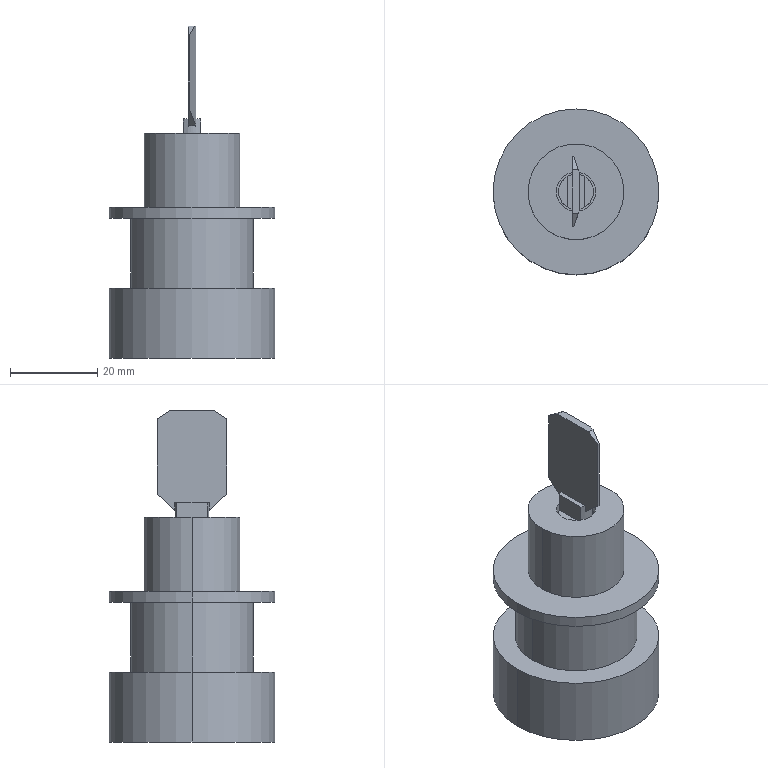Part | SolidWorks | features Boss 6, Chamfer 2, 3DProfileFeature 1, Cut 1, Extrusion 1, HoleWzd 1 | 1 solid | 35 faces | box 38 x 38 x 76.09 mm | volume 37798 mm3 | plane 23 | cylinder 12 | commonest cylinder face diameters 38 x4 8 x2 9 x2 22 x2 28 x2
STEP:
#1=CARTESIAN_POINT('',(4.,0.,50.5));
#2=VERTEX_POINT('',#1);
#3=CARTESIAN_POINT('',(2.,3.464,50.5));
#4=VERTEX_POINT('',#3);
#5=CARTESIAN_POINT('',(0.,0.,50.5));
#6=DIRECTION('',(0.,0.,1.));
#7=DIRECTION('',(1.,0.,0.));
#8=AXIS2_PLACEMENT_3D('',#5,#6,#7);
#9=CIRCLE('',#8,4.);
#10=EDGE_CURVE('',#2,#4,#9,.T.);
#11=ORIENTED_EDGE('',*,*,#10,.F.);
#12=CARTESIAN_POINT('',(4.,0.,46.5));
#13=VERTEX_POINT('',#12);
#14=CARTESIAN_POINT('',(4.,0.,50.5));
#15=DIRECTION('',(0.,0.,-1.));
#16=VECTOR('',#15,1000.);
#17=LINE('',#14,#16);
#18=EDGE_CURVE('',#2,#13,#17,.T.);
#19=ORIENTED_EDGE('',*,*,#18,.T.);
#20=CARTESIAN_POINT('',(-4.,0.,46.5));
#21=VERTEX_POINT('',#20);
#22=CARTESIAN_POINT('',(0.,0.,46.5));
#23=DIRECTION('',(0.,0.,1.));
#24=DIRECTION('',(-1.,0.,0.));
#25=AXIS2_PLACEMENT_3D('',#22,#23,#24);
#26=CIRCLE('',#25,4.);
#27=EDGE_CURVE('',#13,#21,#26,.T.);
#28=ORIENTED_EDGE('',*,*,#27,.T.);
#29=CARTESIAN_POINT('',(-4.,0.,50.5));
#30=VERTEX_POINT('',#29);
#31=CARTESIAN_POINT('',(-4.,0.,50.5));
#32=DIRECTION('',(0.,0.,-1.));
#33=VECTOR('',#32,1000.);
#34=LINE('',#31,#33);
#35=EDGE_CURVE('',#30,#21,#34,.T.);
#36=ORIENTED_EDGE('',*,*,#35,.F.);
#37=CARTESIAN_POINT('',(-2.,3.464,50.5));
#38=VERTEX_POINT('',#37);
#39=CARTESIAN_POINT('',(0.,0.,50.5));
#40=DIRECTION('',(0.,0.,1.));
#41=DIRECTION('',(1.,0.,0.));
#42=AXIS2_PLACEMENT_3D('',#39,#40,#41);
#43=CIRCLE('',#42,4.);
#44=EDGE_CURVE('',#38,#30,#43,.T.);
#45=ORIENTED_EDGE('',*,*,#44,.F.);
#46=CARTESIAN_POINT('',(-2.,3.464,54.8));
#47=VERTEX_POINT('',#46);
#48=CARTESIAN_POINT('',(-2.,3.464,54.8));
#49=DIRECTION('',(0.,0.,-1.));
#50=VECTOR('',#49,1000.);
#51=LINE('',#48,#50);
#52=EDGE_CURVE('',#47,#38,#51,.T.);
#53=ORIENTED_EDGE('',*,*,#52,.F.);
#54=CARTESIAN_POINT('',(-0.9,3.897,54.8));
#55=VERTEX_POINT('',#54);
#56=CARTESIAN_POINT('',(0.,0.,54.8));
#57=DIRECTION('',(0.,0.,1.));
#58=DIRECTION('',(1.,0.,0.));
#59=AXIS2_PLACEMENT_3D('',#56,#57,#58);
#60=CIRCLE('',#59,4.);
#61=EDGE_CURVE('',#55,#47,#60,.T.);
#62=ORIENTED_EDGE('',*,*,#61,.F.);
#63=CARTESIAN_POINT('',(-0.9,3.897,53.153));
#64=VERTEX_POINT('',#63);
#65=CARTESIAN_POINT('',(-0.9,3.897,52.8));
#66=DIRECTION('',(0.,0.,1.));
#67=VECTOR('',#66,1000.);
#68=LINE('',#65,#67);
#69=EDGE_CURVE('',#64,#55,#68,.T.);
#70=ORIENTED_EDGE('',*,*,#69,.F.);
#71=CARTESIAN_POINT('',(0.9,3.897,53.153));
#72=VERTEX_POINT('',#71);
#73=CARTESIAN_POINT('',(-0.9,3.897,53.153));
#74=CARTESIAN_POINT('',(-0.3052,4.035,53.275));
#75=CARTESIAN_POINT('',(0.3052,4.035,53.275));
#76=CARTESIAN_POINT('',(0.9,3.897,53.153));
#77=(BOUNDED_CURVE()B_SPLINE_CURVE(3,(#73,#74,#75,#76),.UNSPECIFIED.,.F.,.F.)B_SPLINE_CURVE_WITH_KNOTS((4,4),(2.915,3.369),.UNSPECIFIED.)CURVE()GEOMETRIC_REPRESENTATION_ITEM()RATIONAL_B_SPLINE_CURVE((1.,0.9829,0.9829,1.))REPRESENTATION_ITEM(''));
#78=EDGE_CURVE('',#64,#72,#77,.T.);
#79=ORIENTED_EDGE('',*,*,#78,.T.);
#80=CARTESIAN_POINT('',(0.9,3.897,54.8));
#81=VERTEX_POINT('',#80);
#82=CARTESIAN_POINT('',(0.9,3.897,52.8));
#83=DIRECTION('',(0.,0.,1.));
#84=VECTOR('',#83,1000.);
#85=LINE('',#82,#84);
#86=EDGE_CURVE('',#72,#81,#85,.T.);
#87=ORIENTED_EDGE('',*,*,#86,.T.);
#88=CARTESIAN_POINT('',(2.,3.464,54.8));
#89=VERTEX_POINT('',#88);
#90=CARTESIAN_POINT('',(0.,0.,54.8));
#91=DIRECTION('',(0.,0.,1.));
#92=DIRECTION('',(1.,0.,0.));
#93=AXIS2_PLACEMENT_3D('',#90,#91,#92);
#94=CIRCLE('',#93,4.);
#95=EDGE_CURVE('',#89,#81,#94,.T.);
#96=ORIENTED_EDGE('',*,*,#95,.F.);
#97=CARTESIAN_POINT('',(2.,3.464,54.8));
#98=DIRECTION('',(0.,0.,-1.));
#99=VECTOR('',#98,1000.);
#100=LINE('',#97,#99);
#101=EDGE_CURVE('',#89,#4,#100,.T.);
#102=ORIENTED_EDGE('',*,*,#101,.T.);
#103=EDGE_LOOP('',(#11,#19,#28,#36,#45,#53,#62,#70,#79,#87,#96,#102));
#104=FACE_OUTER_BOUND('',#103,.T.);
#105=CARTESIAN_POINT('',(0.,0.,50.5));
#106=DIRECTION('',(0.,0.,-1.));
#107=DIRECTION('',(-1.,0.,0.));
#108=AXIS2_PLACEMENT_3D('',#105,#106,#107);
#109=CYLINDRICAL_SURFACE('',#108,4.);
#110=ADVANCED_FACE('',(#104),#109,.T.);
#111=CARTESIAN_POINT('',(-4.5,0.,46.5));
#112=VERTEX_POINT('',#111);
#113=CARTESIAN_POINT('',(4.5,0.,46.5));
#114=VERTEX_POINT('',#113);
#115=CARTESIAN_POINT('',(0.,0.,46.5));
#116=DIRECTION('',(0.,0.,1.));
#117=DIRECTION('',(1.,0.,0.));
#118=AXIS2_PLACEMENT_3D('',#115,#116,#117);
#119=CIRCLE('',#118,4.5);
#120=EDGE_CURVE('',#112,#114,#119,.T.);
#121=ORIENTED_EDGE('',*,*,#120,.F.);
#122=CARTESIAN_POINT('',(-4.5,0.,51.5));
#123=VERTEX_POINT('',#122);
#124=CARTESIAN_POINT('',(-4.5,0.,51.5));
#125=DIRECTION('',(0.,0.,1.));
#126=VECTOR('',#125,1000.);
#127=LINE('',#124,#126);
#128=EDGE_CURVE('',#112,#123,#127,.T.);
#129=ORIENTED_EDGE('',*,*,#128,.T.);
#130=CARTESIAN_POINT('',(4.5,0.,51.5));
#131=VERTEX_POINT('',#130);
#132=CARTESIAN_POINT('',(0.,0.,51.5));
#133=DIRECTION('',(0.,0.,1.));
#134=DIRECTION('',(1.,0.,0.));
#135=AXIS2_PLACEMENT_3D('',#132,#133,#134);
#136=CIRCLE('',#135,4.5);
#137=EDGE_CURVE('',#123,#131,#136,.T.);
#138=ORIENTED_EDGE('',*,*,#137,.T.);
#139=CARTESIAN_POINT('',(4.5,0.,51.5));
#140=DIRECTION('',(0.,0.,1.));
#141=VECTOR('',#140,1000.);
#142=LINE('',#139,#141);
#143=EDGE_CURVE('',#114,#131,#142,.T.);
#144=ORIENTED_EDGE('',*,*,#143,.F.);
#145=EDGE_LOOP('',(#121,#129,#138,#144));
#146=FACE_OUTER_BOUND('',#145,.T.);
#147=CARTESIAN_POINT('',(0.,0.,51.5));
#148=DIRECTION('',(0.,0.,1.));
#149=DIRECTION('',(1.,0.,0.));
#150=AXIS2_PLACEMENT_3D('',#147,#148,#149);
#151=CYLINDRICAL_SURFACE('',#150,4.5);
#152=ADVANCED_FACE('',(#146),#151,.F.);
#153=CARTESIAN_POINT('',(11.,0.,51.5));
#154=VERTEX_POINT('',#153);
#155=CARTESIAN_POINT('',(-11.,0.,51.5));
#156=VERTEX_POINT('',#155);
#157=CARTESIAN_POINT('',(0.,0.,51.5));
#158=DIRECTION('',(0.,0.,1.));
#159=DIRECTION('',(1.,0.,0.));
#160=AXIS2_PLACEMENT_3D('',#157,#158,#159);
#161=CIRCLE('',#160,11.);
#162=EDGE_CURVE('',#154,#156,#161,.T.);
#163=ORIENTED_EDGE('',*,*,#162,.F.);
#164=CARTESIAN_POINT('',(11.,0.,34.5));
#165=VERTEX_POINT('',#164);
#166=CARTESIAN_POINT('',(11.,0.,51.5));
#167=DIRECTION('',(0.,0.,-1.));
#168=VECTOR('',#167,1000.);
#169=LINE('',#166,#168);
#170=EDGE_CURVE('',#154,#165,#169,.T.);
#171=ORIENTED_EDGE('',*,*,#170,.T.);
#172=CARTESIAN_POINT('',(-11.,0.,34.5));
#173=VERTEX_POINT('',#172);
#174=CARTESIAN_POINT('',(0.,0.,34.5));
#175=DIRECTION('',(0.,0.,1.));
#176=DIRECTION('',(1.,0.,0.));
#177=AXIS2_PLACEMENT_3D('',#174,#175,#176);
#178=CIRCLE('',#177,11.);
#179=EDGE_CURVE('',#165,#173,#178,.T.);
#180=ORIENTED_EDGE('',*,*,#179,.T.);
#181=CARTESIAN_POINT('',(-11.,0.,51.5));
#182=DIRECTION('',(0.,0.,-1.));
#183=VECTOR('',#182,1000.);
#184=LINE('',#181,#183);
#185=EDGE_CURVE('',#156,#173,#184,.T.);
#186=ORIENTED_EDGE('',*,*,#185,.F.);
#187=EDGE_LOOP('',(#163,#171,#180,#186));
#188=FACE_OUTER_BOUND('',#187,.T.);
#189=CARTESIAN_POINT('',(0.,0.,51.5));
#190=DIRECTION('',(0.,0.,-1.));
#191=DIRECTION('',(-1.,0.,0.));
#192=AXIS2_PLACEMENT_3D('',#189,#190,#191);
#193=CYLINDRICAL_SURFACE('',#192,11.);
#194=ADVANCED_FACE('',(#188),#193,.T.);
#195=CARTESIAN_POINT('',(19.,0.,34.5));
#196=VERTEX_POINT('',#195);
#197=CARTESIAN_POINT('',(-19.,0.,34.5));
#198=VERTEX_POINT('',#197);
#199=CARTESIAN_POINT('',(0.,0.,34.5));
#200=DIRECTION('',(0.,0.,1.));
#201=DIRECTION('',(1.,0.,0.));
#202=AXIS2_PLACEMENT_3D('',#199,#200,#201);
#203=CIRCLE('',#202,19.);
#204=EDGE_CURVE('',#196,#198,#203,.T.);
#205=ORIENTED_EDGE('',*,*,#204,.F.);
#206=CARTESIAN_POINT('',(19.,0.,32.));
#207=VERTEX_POINT('',#206);
#208=CARTESIAN_POINT('',(19.,0.,34.5));
#209=DIRECTION('',(0.,0.,-1.));
#210=VECTOR('',#209,1000.);
#211=LINE('',#208,#210);
#212=EDGE_CURVE('',#196,#207,#211,.T.);
#213=ORIENTED_EDGE('',*,*,#212,.T.);
#214=CARTESIAN_POINT('',(-19.,0.,32.));
#215=VERTEX_POINT('',#214);
#216=CARTESIAN_POINT('',(0.,0.,32.));
#217=DIRECTION('',(0.,0.,1.));
#218=DIRECTION('',(1.,0.,0.));
#219=AXIS2_PLACEMENT_3D('',#216,#217,#218);
#220=CIRCLE('',#219,19.);
#221=EDGE_CURVE('',#207,#215,#220,.T.);
#222=ORIENTED_EDGE('',*,*,#221,.T.);
#223=CARTESIAN_POINT('',(-19.,0.,34.5));
#224=DIRECTION('',(0.,0.,-1.));
#225=VECTOR('',#224,1000.);
#226=LINE('',#223,#225);
#227=EDGE_CURVE('',#198,#215,#226,.T.);
#228=ORIENTED_EDGE('',*,*,#227,.F.);
#229=EDGE_LOOP('',(#205,#213,#222,#228));
#230=FACE_OUTER_BOUND('',#229,.T.);
#231=CARTESIAN_POINT('',(0.,0.,34.5));
#232=DIRECTION('',(0.,0.,-1.));
#233=DIRECTION('',(-1.,0.,0.));
#234=AXIS2_PLACEMENT_3D('',#231,#232,#233);
#235=CYLINDRICAL_SURFACE('',#234,19.);
#236=ADVANCED_FACE('',(#230),#235,.T.);
#237=CARTESIAN_POINT('',(14.,0.,32.));
#238=VERTEX_POINT('',#237);
#239=CARTESIAN_POINT('',(-14.,0.,32.));
#240=VERTEX_POINT('',#239);
#241=CARTESIAN_POINT('',(0.,0.,32.));
#242=DIRECTION('',(0.,0.,1.));
#243=DIRECTION('',(1.,0.,0.));
#244=AXIS2_PLACEMENT_3D('',#241,#242,#243);
#245=CIRCLE('',#244,14.);
#246=EDGE_CURVE('',#238,#240,#245,.T.);
#247=ORIENTED_EDGE('',*,*,#246,.F.);
#248=CARTESIAN_POINT('',(14.,0.,16.));
#249=VERTEX_POINT('',#248);
#250=CARTESIAN_POINT('',(14.,0.,32.));
#251=DIRECTION('',(0.,0.,-1.));
#252=VECTOR('',#251,1000.);
#253=LINE('',#250,#252);
#254=EDGE_CURVE('',#238,#249,#253,.T.);
#255=ORIENTED_EDGE('',*,*,#254,.T.);
#256=CARTESIAN_POINT('',(-14.,0.,16.));
#257=VERTEX_POINT('',#256);
#258=CARTESIAN_POINT('',(0.,0.,16.));
#259=DIRECTION('',(0.,0.,1.));
#260=DIRECTION('',(1.,0.,0.));
#261=AXIS2_PLACEMENT_3D('',#258,#259,#260);
#262=CIRCLE('',#261,14.);
#263=EDGE_CURVE('',#249,#257,#262,.T.);
#264=ORIENTED_EDGE('',*,*,#263,.T.);
#265=CARTESIAN_POINT('',(-14.,0.,32.));
#266=DIRECTION('',(0.,0.,-1.));
#267=VECTOR('',#266,1000.);
#268=LINE('',#265,#267);
#269=EDGE_CURVE('',#240,#257,#268,.T.);
#270=ORIENTED_EDGE('',*,*,#269,.F.);
#271=EDGE_LOOP('',(#247,#255,#264,#270));
#272=FACE_OUTER_BOUND('',#271,.T.);
#273=CARTESIAN_POINT('',(0.,0.,32.));
#274=DIRECTION('',(0.,0.,-1.));
#275=DIRECTION('',(-1.,0.,0.));
#276=AXIS2_PLACEMENT_3D('',#273,#274,#275);
#277=CYLINDRICAL_SURFACE('',#276,14.);
#278=ADVANCED_FACE('',(#272),#277,.T.);
#279=CARTESIAN_POINT('',(19.,0.,16.));
#280=VERTEX_POINT('',#279);
#281=CARTESIAN_POINT('',(-19.,0.,16.));
#282=VERTEX_POINT('',#281);
#283=CARTESIAN_POINT('',(0.,0.,16.));
#284=DIRECTION('',(0.,0.,1.));
#285=DIRECTION('',(1.,0.,0.));
#286=AXIS2_PLACEMENT_3D('',#283,#284,#285);
#287=CIRCLE('',#286,19.);
#288=EDGE_CURVE('',#280,#282,#287,.T.);
#289=ORIENTED_EDGE('',*,*,#288,.F.);
#290=CARTESIAN_POINT('',(19.,0.,0.));
#291=VERTEX_POINT('',#290);
#292=CARTESIAN_POINT('',(19.,0.,16.));
#293=DIRECTION('',(0.,0.,-1.));
#294=VECTOR('',#293,1000.);
#295=LINE('',#292,#294);
#296=EDGE_CURVE('',#280,#291,#295,.T.);
#297=ORIENTED_EDGE('',*,*,#296,.T.);
#298=CARTESIAN_POINT('',(-19.,0.,0.));
#299=VERTEX_POINT('',#298);
#300=CARTESIAN_POINT('',(0.,0.,0.));
#301=DIRECTION('',(0.,0.,1.));
#302=DIRECTION('',(1.,0.,0.));
#303=AXIS2_PLACEMENT_3D('',#300,#301,#302);
#304=CIRCLE('',#303,19.);
#305=EDGE_CURVE('',#291,#299,#304,.T.);
#306=ORIENTED_EDGE('',*,*,#305,.T.);
#307=CARTESIAN_POINT('',(-19.,0.,16.));
#308=DIRECTION('',(0.,0.,-1.));
#309=VECTOR('',#308,1000.);
#310=LINE('',#307,#309);
#311=EDGE_CURVE('',#282,#299,#310,.T.);
#312=ORIENTED_EDGE('',*,*,#311,.F.);
#313=EDGE_LOOP('',(#289,#297,#306,#312));
#314=FACE_OUTER_BOUND('',#313,.T.);
#315=CARTESIAN_POINT('',(0.,0.,16.));
#316=DIRECTION('',(0.,0.,-1.));
#317=DIRECTION('',(-1.,0.,0.));
#318=AXIS2_PLACEMENT_3D('',#315,#316,#317);
#319=CYLINDRICAL_SURFACE('',#318,19.);
#320=ADVANCED_FACE('',(#314),#319,.T.);
#321=CARTESIAN_POINT('',(0.9,-3.897,54.8));
#322=VERTEX_POINT('',#321);
#323=CARTESIAN_POINT('',(0.9,3.897,54.8));
#324=DIRECTION('',(0.,1.,0.));
#325=VECTOR('',#324,1000.);
#326=LINE('',#323,#325);
#327=EDGE_CURVE('',#322,#81,#326,.T.);
#328=ORIENTED_EDGE('',*,*,#327,.F.);
#329=CARTESIAN_POINT('',(2.,-3.464,54.8));
#330=VERTEX_POINT('',#329);
#331=CARTESIAN_POINT('',(0.,0.,54.8));
#332=DIRECTION('',(0.,0.,1.));
#333=DIRECTION('',(1.,0.,0.));
#334=AXIS2_PLACEMENT_3D('',#331,#332,#333);
#335=CIRCLE('',#334,4.);
#336=EDGE_CURVE('',#322,#330,#335,.T.);
#337=ORIENTED_EDGE('',*,*,#336,.T.);
#338=CARTESIAN_POINT('',(2.,3.464,54.8));
#339=DIRECTION('',(0.,1.,0.));
#340=VECTOR('',#339,1000.);
#341=LINE('',#338,#340);
#342=EDGE_CURVE('',#330,#89,#341,.T.);
#343=ORIENTED_EDGE('',*,*,#342,.T.);
#344=ORIENTED_EDGE('',*,*,#95,.T.);
#345=EDGE_LOOP('',(#328,#337,#343,#344));
#346=FACE_OUTER_BOUND('',#345,.T.);
#347=CARTESIAN_POINT('',(0.,0.,54.8));
#348=DIRECTION('',(0.,0.,1.));
#349=DIRECTION('',(1.,0.,0.));
#350=AXIS2_PLACEMENT_3D('',#347,#348,#349);
#351=PLANE('',#350);
#352=ADVANCED_FACE('',(#346),#351,.T.);
#353=CARTESIAN_POINT('',(2.,-3.464,50.5));
#354=VERTEX_POINT('',#353);
#355=CARTESIAN_POINT('',(2.,3.464,50.5));
#356=DIRECTION('',(0.,1.,0.));
#357=VECTOR('',#356,1000.);
#358=LINE('',#355,#357);
#359=EDGE_CURVE('',#354,#4,#358,.T.);
#360=ORIENTED_EDGE('',*,*,#359,.F.);
#361=CARTESIAN_POINT('',(0.,0.,50.5));
#362=DIRECTION('',(0.,0.,1.));
#363=DIRECTION('',(1.,0.,0.));
#364=AXIS2_PLACEMENT_3D('',#361,#362,#363);
#365=CIRCLE('',#364,4.);
#366=EDGE_CURVE('',#354,#2,#365,.T.);
#367=ORIENTED_EDGE('',*,*,#366,.T.);
#368=ORIENTED_EDGE('',*,*,#10,.T.);
#369=EDGE_LOOP('',(#360,#367,#368));
#370=FACE_OUTER_BOUND('',#369,.T.);
#371=CARTESIAN_POINT('',(0.,0.,50.5));
#372=DIRECTION('',(0.,0.,1.));
#373=DIRECTION('',(1.,0.,0.));
#374=AXIS2_PLACEMENT_3D('',#371,#372,#373);
#375=PLANE('',#374);
#376=ADVANCED_FACE('',(#370),#375,.T.);
#377=CARTESIAN_POINT('',(0.,0.,46.5));
#378=DIRECTION('',(0.,0.,1.));
#379=DIRECTION('',(1.,0.,0.));
#380=AXIS2_PLACEMENT_3D('',#377,#378,#379);
#381=CIRCLE('',#380,4.5);
#382=EDGE_CURVE('',#114,#112,#381,.T.);
#383=ORIENTED_EDGE('',*,*,#382,.T.);
#384=ORIENTED_EDGE('',*,*,#120,.T.);
#385=EDGE_LOOP('',(#383,#384));
#386=FACE_OUTER_BOUND('',#385,.T.);
#387=CARTESIAN_POINT('',(0.,0.,46.5));
#388=DIRECTION('',(0.,0.,1.));
#389=DIRECTION('',(-1.,0.,0.));
#390=AXIS2_PLACEMENT_3D('',#387,#388,#389);
#391=CIRCLE('',#390,4.);
#392=EDGE_CURVE('',#21,#13,#391,.T.);
#393=ORIENTED_EDGE('',*,*,#392,.F.);
#394=ORIENTED_EDGE('',*,*,#27,.F.);
#395=EDGE_LOOP('',(#393,#394));
#396=FACE_BOUND('',#395,.T.);
#397=CARTESIAN_POINT('',(0.,0.,46.5));
#398=DIRECTION('',(0.,0.,-1.));
#399=DIRECTION('',(-1.,0.,0.));
#400=AXIS2_PLACEMENT_3D('',#397,#398,#399);
#401=PLANE('',#400);
#402=ADVANCED_FACE('',(#386,#396),#401,.F.);
#403=CARTESIAN_POINT('',(0.,0.,34.5));
#404=DIRECTION('',(0.,0.,1.));
#405=DIRECTION('',(1.,0.,0.));
#406=AXIS2_PLACEMENT_3D('',#403,#404,#405);
#407=CIRCLE('',#406,19.);
#408=EDGE_CURVE('',#198,#196,#407,.T.);
#409=ORIENTED_EDGE('',*,*,#408,.T.);
#410=ORIENTED_EDGE('',*,*,#204,.T.);
#411=EDGE_LOOP('',(#409,#410));
#412=FACE_OUTER_BOUND('',#411,.T.);
#413=CARTESIAN_POINT('',(0.,0.,34.5));
#414=DIRECTION('',(0.,0.,1.));
#415=DIRECTION('',(1.,0.,0.));
#416=AXIS2_PLACEMENT_3D('',#413,#414,#415);
#417=CIRCLE('',#416,11.);
#418=EDGE_CURVE('',#173,#165,#417,.T.);
#419=ORIENTED_EDGE('',*,*,#418,.F.);
#420=ORIENTED_EDGE('',*,*,#179,.F.);
#421=EDGE_LOOP('',(#419,#420));
#422=FACE_BOUND('',#421,.T.);
#423=CARTESIAN_POINT('',(0.,0.,34.5));
#424=DIRECTION('',(0.,0.,1.));
#425=DIRECTION('',(1.,0.,0.));
#426=AXIS2_PLACEMENT_3D('',#423,#424,#425);
#427=PLANE('',#426);
#428=ADVANCED_FACE('',(#412,#422),#427,.T.);
#429=CARTESIAN_POINT('',(0.,0.,16.));
#430=DIRECTION('',(0.,0.,1.));
#431=DIRECTION('',(1.,0.,0.));
#432=AXIS2_PLACEMENT_3D('',#429,#430,#431);
#433=CIRCLE('',#432,19.);
#434=EDGE_CURVE('',#282,#280,#433,.T.);
#435=ORIENTED_EDGE('',*,*,#434,.T.);
#436=ORIENTED_EDGE('',*,*,#288,.T.);
#437=EDGE_LOOP('',(#435,#436));
#438=FACE_OUTER_BOUND('',#437,.T.);
#439=CARTESIAN_POINT('',(0.,0.,16.));
#440=DIRECTION('',(0.,0.,1.));
#441=DIRECTION('',(1.,0.,0.));
#442=AXIS2_PLACEMENT_3D('',#439,#440,#441);
#443=CIRCLE('',#442,14.);
#444=EDGE_CURVE('',#257,#249,#443,.T.);
#445=ORIENTED_EDGE('',*,*,#444,.F.);
#446=ORIENTED_EDGE('',*,*,#263,.F.);
#447=EDGE_LOOP('',(#445,#446));
#448=FACE_BOUND('',#447,.T.);
#449=CARTESIAN_POINT('',(0.,0.,16.));
#450=DIRECTION('',(0.,0.,1.));
#451=DIRECTION('',(1.,0.,0.));
#452=AXIS2_PLACEMENT_3D('',#449,#450,#451);
#453=PLANE('',#452);
#454=ADVANCED_FACE('',(#438,#448),#453,.T.);
#455=ORIENTED_EDGE('',*,*,#296,.F.);
#456=ORIENTED_EDGE('',*,*,#434,.F.);
#457=ORIENTED_EDGE('',*,*,#311,.T.);
#458=CARTESIAN_POINT('',(0.,0.,0.));
#459=DIRECTION('',(0.,0.,1.));
#460=DIRECTION('',(1.,0.,0.));
#461=AXIS2_PLACEMENT_3D('',#458,#459,#460);
#462=CIRCLE('',#461,19.);
#463=EDGE_CURVE('',#299,#291,#462,.T.);
#464=ORIENTED_EDGE('',*,*,#463,.T.);
#465=EDGE_LOOP('',(#455,#456,#457,#464));
#466=FACE_OUTER_BOUND('',#465,.T.);
#467=CARTESIAN_POINT('',(0.,0.,16.));
#468=DIRECTION('',(0.,0.,-1.));
#469=DIRECTION('',(-1.,0.,0.));
#470=AXIS2_PLACEMENT_3D('',#467,#468,#469);
#471=CYLINDRICAL_SURFACE('',#470,19.);
#472=ADVANCED_FACE('',(#466),#471,.T.);
#473=ORIENTED_EDGE('',*,*,#463,.F.);
#474=ORIENTED_EDGE('',*,*,#305,.F.);
#475=EDGE_LOOP('',(#473,#474));
#476=FACE_OUTER_BOUND('',#475,.T.);
#477=CARTESIAN_POINT('',(0.,0.,0.));
#478=DIRECTION('',(0.,0.,1.));
#479=DIRECTION('',(1.,0.,0.));
#480=AXIS2_PLACEMENT_3D('',#477,#478,#479);
#481=PLANE('',#480);
#482=ADVANCED_FACE('',(#476),#481,.F.);
#483=ORIENTED_EDGE('',*,*,#254,.F.);
#484=CARTESIAN_POINT('',(0.,0.,32.));
#485=DIRECTION('',(0.,0.,1.));
#486=DIRECTION('',(1.,0.,0.));
#487=AXIS2_PLACEMENT_3D('',#484,#485,#486);
#488=CIRCLE('',#487,14.);
#489=EDGE_CURVE('',#240,#238,#488,.T.);
#490=ORIENTED_EDGE('',*,*,#489,.F.);
#491=ORIENTED_EDGE('',*,*,#269,.T.);
#492=ORIENTED_EDGE('',*,*,#444,.T.);
#493=EDGE_LOOP('',(#483,#490,#491,#492));
#494=FACE_OUTER_BOUND('',#493,.T.);
#495=CARTESIAN_POINT('',(0.,0.,32.));
#496=DIRECTION('',(0.,0.,-1.));
#497=DIRECTION('',(-1.,0.,0.));
#498=AXIS2_PLACEMENT_3D('',#495,#496,#497);
#499=CYLINDRICAL_SURFACE('',#498,14.);
#500=ADVANCED_FACE('',(#494),#499,.T.);
#501=CARTESIAN_POINT('',(0.,0.,32.));
#502=DIRECTION('',(0.,0.,1.));
#503=DIRECTION('',(1.,0.,0.));
#504=AXIS2_PLACEMENT_3D('',#501,#502,#503);
#505=CIRCLE('',#504,19.);
#506=EDGE_CURVE('',#215,#207,#505,.T.);
#507=ORIENTED_EDGE('',*,*,#506,.F.);
#508=ORIENTED_EDGE('',*,*,#221,.F.);
#509=EDGE_LOOP('',(#507,#508));
#510=FACE_OUTER_BOUND('',#509,.T.);
#511=ORIENTED_EDGE('',*,*,#489,.T.);
#512=ORIENTED_EDGE('',*,*,#246,.T.);
#513=EDGE_LOOP('',(#511,#512));
#514=FACE_BOUND('',#513,.T.);
#515=CARTESIAN_POINT('',(0.,0.,32.));
#516=DIRECTION('',(0.,0.,1.));
#517=DIRECTION('',(1.,0.,0.));
#518=AXIS2_PLACEMENT_3D('',#515,#516,#517);
#519=PLANE('',#518);
#520=ADVANCED_FACE('',(#510,#514),#519,.F.);
#521=ORIENTED_EDGE('',*,*,#212,.F.);
#522=ORIENTED_EDGE('',*,*,#408,.F.);
#523=ORIENTED_EDGE('',*,*,#227,.T.);
#524=ORIENTED_EDGE('',*,*,#506,.T.);
#525=EDGE_LOOP('',(#521,#522,#523,#524));
#526=FACE_OUTER_BOUND('',#525,.T.);
#527=CARTESIAN_POINT('',(0.,0.,34.5));
#528=DIRECTION('',(0.,0.,-1.));
#529=DIRECTION('',(-1.,0.,0.));
#530=AXIS2_PLACEMENT_3D('',#527,#528,#529);
#531=CYLINDRICAL_SURFACE('',#530,19.);
#532=ADVANCED_FACE('',(#526),#531,.T.);
#533=ORIENTED_EDGE('',*,*,#170,.F.);
#534=CARTESIAN_POINT('',(0.,0.,51.5));
#535=DIRECTION('',(0.,0.,1.));
#536=DIRECTION('',(1.,0.,0.));
#537=AXIS2_PLACEMENT_3D('',#534,#535,#536);
#538=CIRCLE('',#537,11.);
#539=EDGE_CURVE('',#156,#154,#538,.T.);
#540=ORIENTED_EDGE('',*,*,#539,.F.);
#541=ORIENTED_EDGE('',*,*,#185,.T.);
#542=ORIENTED_EDGE('',*,*,#418,.T.);
#543=EDGE_LOOP('',(#533,#540,#541,#542));
#544=FACE_OUTER_BOUND('',#543,.T.);
#545=CARTESIAN_POINT('',(0.,0.,51.5));
#546=DIRECTION('',(0.,0.,-1.));
#547=DIRECTION('',(-1.,0.,0.));
#548=AXIS2_PLACEMENT_3D('',#545,#546,#547);
#549=CYLINDRICAL_SURFACE('',#548,11.);
#550=ADVANCED_FACE('',(#544),#549,.T.);
#551=CARTESIAN_POINT('',(0.,0.,51.5));
#552=DIRECTION('',(0.,0.,1.));
#553=DIRECTION('',(1.,0.,0.));
#554=AXIS2_PLACEMENT_3D('',#551,#552,#553);
#555=CIRCLE('',#554,4.5);
#556=EDGE_CURVE('',#131,#123,#555,.T.);
#557=ORIENTED_EDGE('',*,*,#556,.F.);
#558=ORIENTED_EDGE('',*,*,#137,.F.);
#559=EDGE_LOOP('',(#557,#558));
#560=FACE_BOUND('',#559,.T.);
#561=ORIENTED_EDGE('',*,*,#539,.T.);
#562=ORIENTED_EDGE('',*,*,#162,.T.);
#563=EDGE_LOOP('',(#561,#562));
#564=FACE_OUTER_BOUND('',#563,.T.);
#565=CARTESIAN_POINT('',(0.,0.,51.5));
#566=DIRECTION('',(0.,0.,1.));
#567=DIRECTION('',(1.,0.,0.));
#568=AXIS2_PLACEMENT_3D('',#565,#566,#567);
#569=PLANE('',#568);
#570=ADVANCED_FACE('',(#560,#564),#569,.T.);
#571=ORIENTED_EDGE('',*,*,#128,.F.);
#572=ORIENTED_EDGE('',*,*,#382,.F.);
#573=ORIENTED_EDGE('',*,*,#143,.T.);
#574=ORIENTED_EDGE('',*,*,#556,.T.);
#575=EDGE_LOOP('',(#571,#572,#573,#574));
#576=FACE_OUTER_BOUND('',#575,.T.);
#577=CARTESIAN_POINT('',(0.,0.,51.5));
#578=DIRECTION('',(0.,0.,1.));
#579=DIRECTION('',(1.,0.,0.));
#580=AXIS2_PLACEMENT_3D('',#577,#578,#579);
#581=CYLINDRICAL_SURFACE('',#580,4.5);
#582=ADVANCED_FACE('',(#576),#581,.F.);
#583=ORIENTED_EDGE('',*,*,#18,.F.);
#584=ORIENTED_EDGE('',*,*,#366,.F.);
#585=CARTESIAN_POINT('',(2.,-3.464,54.8));
#586=DIRECTION('',(0.,0.,-1.));
#587=VECTOR('',#586,1000.);
#588=LINE('',#585,#587);
#589=EDGE_CURVE('',#330,#354,#588,.T.);
#590=ORIENTED_EDGE('',*,*,#589,.F.);
#591=ORIENTED_EDGE('',*,*,#336,.F.);
#592=CARTESIAN_POINT('',(0.9,-3.897,53.153));
#593=VERTEX_POINT('',#592);
#594=CARTESIAN_POINT('',(0.9,-3.897,52.8));
#595=DIRECTION('',(0.,0.,1.));
#596=VECTOR('',#595,1000.);
#597=LINE('',#594,#596);
#598=EDGE_CURVE('',#593,#322,#597,.T.);
#599=ORIENTED_EDGE('',*,*,#598,.F.);
#600=CARTESIAN_POINT('',(-0.9,-3.897,53.153));
#601=VERTEX_POINT('',#600);
#602=CARTESIAN_POINT('',(0.9,-3.897,53.153));
#603=CARTESIAN_POINT('',(0.3052,-4.035,53.275));
#604=CARTESIAN_POINT('',(-0.3052,-4.035,53.275));
#605=CARTESIAN_POINT('',(-0.9,-3.897,53.153));
#606=(BOUNDED_CURVE()B_SPLINE_CURVE(3,(#602,#603,#604,#605),.UNSPECIFIED.,.F.,.F.)B_SPLINE_CURVE_WITH_KNOTS((4,4),(2.915,3.369),.UNSPECIFIED.)CURVE()GEOMETRIC_REPRESENTATION_ITEM()RATIONAL_B_SPLINE_CURVE((1.,0.9829,0.9829,1.))REPRESENTATION_ITEM(''));
#607=EDGE_CURVE('',#593,#601,#606,.T.);
#608=ORIENTED_EDGE('',*,*,#607,.T.);
#609=CARTESIAN_POINT('',(-0.9,-3.897,54.8));
#610=VERTEX_POINT('',#609);
#611=CARTESIAN_POINT('',(-0.9,-3.897,52.8));
#612=DIRECTION('',(0.,0.,1.));
#613=VECTOR('',#612,1000.);
#614=LINE('',#611,#613);
#615=EDGE_CURVE('',#601,#610,#614,.T.);
#616=ORIENTED_EDGE('',*,*,#615,.T.);
#617=CARTESIAN_POINT('',(-2.,-3.464,54.8));
#618=VERTEX_POINT('',#617);
#619=CARTESIAN_POINT('',(0.,0.,54.8));
#620=DIRECTION('',(0.,0.,1.));
#621=DIRECTION('',(1.,0.,0.));
#622=AXIS2_PLACEMENT_3D('',#619,#620,#621);
#623=CIRCLE('',#622,4.);
#624=EDGE_CURVE('',#618,#610,#623,.T.);
#625=ORIENTED_EDGE('',*,*,#624,.F.);
#626=CARTESIAN_POINT('',(-2.,-3.464,50.5));
#627=VERTEX_POINT('',#626);
#628=CARTESIAN_POINT('',(-2.,-3.464,54.8));
#629=DIRECTION('',(0.,0.,-1.));
#630=VECTOR('',#629,1000.);
#631=LINE('',#628,#630);
#632=EDGE_CURVE('',#618,#627,#631,.T.);
#633=ORIENTED_EDGE('',*,*,#632,.T.);
#634=CARTESIAN_POINT('',(0.,0.,50.5));
#635=DIRECTION('',(0.,0.,1.));
#636=DIRECTION('',(1.,0.,0.));
#637=AXIS2_PLACEMENT_3D('',#634,#635,#636);
#638=CIRCLE('',#637,4.);
#639=EDGE_CURVE('',#30,#627,#638,.T.);
#640=ORIENTED_EDGE('',*,*,#639,.F.);
#641=ORIENTED_EDGE('',*,*,#35,.T.);
#642=ORIENTED_EDGE('',*,*,#392,.T.);
#643=EDGE_LOOP('',(#583,#584,#590,#591,#599,#608,#616,#625,#633,#640,#641,#642));
#644=FACE_OUTER_BOUND('',#643,.T.);
#645=CARTESIAN_POINT('',(0.,0.,50.5));
#646=DIRECTION('',(0.,0.,-1.));
#647=DIRECTION('',(-1.,0.,0.));
#648=AXIS2_PLACEMENT_3D('',#645,#646,#647);
#649=CYLINDRICAL_SURFACE('',#648,4.);
#650=ADVANCED_FACE('',(#644),#649,.T.);
#651=CARTESIAN_POINT('',(-2.,3.464,50.5));
#652=DIRECTION('',(0.,-1.,0.));
#653=VECTOR('',#652,1000.);
#654=LINE('',#651,#653);
#655=EDGE_CURVE('',#38,#627,#654,.T.);
#656=ORIENTED_EDGE('',*,*,#655,.F.);
#657=ORIENTED_EDGE('',*,*,#44,.T.);
#658=ORIENTED_EDGE('',*,*,#639,.T.);
#659=EDGE_LOOP('',(#656,#657,#658));
#660=FACE_OUTER_BOUND('',#659,.T.);
#661=CARTESIAN_POINT('',(0.,0.,50.5));
#662=DIRECTION('',(0.,0.,1.));
#663=DIRECTION('',(1.,0.,0.));
#664=AXIS2_PLACEMENT_3D('',#661,#662,#663);
#665=PLANE('',#664);
#666=ADVANCED_FACE('',(#660),#665,.T.);
#667=ORIENTED_EDGE('',*,*,#655,.T.);
#668=ORIENTED_EDGE('',*,*,#632,.F.);
#669=CARTESIAN_POINT('',(-2.,3.464,54.8));
#670=DIRECTION('',(0.,-1.,0.));
#671=VECTOR('',#670,1000.);
#672=LINE('',#669,#671);
#673=EDGE_CURVE('',#47,#618,#672,.T.);
#674=ORIENTED_EDGE('',*,*,#673,.F.);
#675=ORIENTED_EDGE('',*,*,#52,.T.);
#676=EDGE_LOOP('',(#667,#668,#674,#675));
#677=FACE_OUTER_BOUND('',#676,.T.);
#678=CARTESIAN_POINT('',(-2.,3.464,54.8));
#679=DIRECTION('',(1.,0.,0.));
#680=DIRECTION('',(0.,1.,0.));
#681=AXIS2_PLACEMENT_3D('',#678,#679,#680);
#682=PLANE('',#681);
#683=ADVANCED_FACE('',(#677),#682,.F.);
#684=ORIENTED_EDGE('',*,*,#359,.T.);
#685=ORIENTED_EDGE('',*,*,#101,.F.);
#686=ORIENTED_EDGE('',*,*,#342,.F.);
#687=ORIENTED_EDGE('',*,*,#589,.T.);
#688=EDGE_LOOP('',(#684,#685,#686,#687));
#689=FACE_OUTER_BOUND('',#688,.T.);
#690=CARTESIAN_POINT('',(2.,3.464,54.8));
#691=DIRECTION('',(-1.,0.,0.));
#692=DIRECTION('',(0.,-1.,0.));
#693=AXIS2_PLACEMENT_3D('',#690,#691,#692);
#694=PLANE('',#693);
#695=ADVANCED_FACE('',(#689),#694,.F.);
#696=CARTESIAN_POINT('',(-0.9,3.897,54.8));
#697=DIRECTION('',(0.,-1.,0.));
#698=VECTOR('',#697,1000.);
#699=LINE('',#696,#698);
#700=EDGE_CURVE('',#55,#610,#699,.T.);
#701=ORIENTED_EDGE('',*,*,#700,.F.);
#702=ORIENTED_EDGE('',*,*,#61,.T.);
#703=ORIENTED_EDGE('',*,*,#673,.T.);
#704=ORIENTED_EDGE('',*,*,#624,.T.);
#705=EDGE_LOOP('',(#701,#702,#703,#704));
#706=FACE_OUTER_BOUND('',#705,.T.);
#707=CARTESIAN_POINT('',(0.,0.,54.8));
#708=DIRECTION('',(0.,0.,1.));
#709=DIRECTION('',(1.,0.,0.));
#710=AXIS2_PLACEMENT_3D('',#707,#708,#709);
#711=PLANE('',#710);
#712=ADVANCED_FACE('',(#706),#711,.T.);
#713=ORIENTED_EDGE('',*,*,#615,.F.);
#714=CARTESIAN_POINT('',(-0.9,-8.,56.8));
#715=VERTEX_POINT('',#714);
#716=CARTESIAN_POINT('',(-0.9,-8.,56.8));
#717=DIRECTION('',(0.,-0.7474,0.6644));
#718=VECTOR('',#717,1000.);
#719=LINE('',#716,#718);
#720=EDGE_CURVE('',#601,#715,#719,.T.);
#721=ORIENTED_EDGE('',*,*,#720,.T.);
#722=CARTESIAN_POINT('',(-0.9,-8.,74.09));
#723=VERTEX_POINT('',#722);
#724=CARTESIAN_POINT('',(-0.9,-8.,76.09));
#725=DIRECTION('',(0.,0.,-1.));
#726=VECTOR('',#725,1000.);
#727=LINE('',#724,#726);
#728=EDGE_CURVE('',#723,#715,#727,.T.);
#729=ORIENTED_EDGE('',*,*,#728,.F.);
#730=CARTESIAN_POINT('',(-0.9,-5.,76.09));
#731=VERTEX_POINT('',#730);
#732=CARTESIAN_POINT('',(-0.9,-5.,76.09));
#733=DIRECTION('',(0.,0.8321,0.5547));
#734=VECTOR('',#733,1000.);
#735=LINE('',#732,#734);
#736=EDGE_CURVE('',#723,#731,#735,.T.);
#737=ORIENTED_EDGE('',*,*,#736,.T.);
#738=CARTESIAN_POINT('',(-0.9,5.,76.09));
#739=VERTEX_POINT('',#738);
#740=CARTESIAN_POINT('',(-0.9,8.,76.09));
#741=DIRECTION('',(0.,-1.,0.));
#742=VECTOR('',#741,1000.);
#743=LINE('',#740,#742);
#744=EDGE_CURVE('',#739,#731,#743,.T.);
#745=ORIENTED_EDGE('',*,*,#744,.F.);
#746=CARTESIAN_POINT('',(-0.9,8.,74.09));
#747=VERTEX_POINT('',#746);
#748=CARTESIAN_POINT('',(-0.9,5.,76.09));
#749=DIRECTION('',(0.,0.8321,-0.5547));
#750=VECTOR('',#749,1000.);
#751=LINE('',#748,#750);
#752=EDGE_CURVE('',#739,#747,#751,.T.);
#753=ORIENTED_EDGE('',*,*,#752,.T.);
#754=CARTESIAN_POINT('',(-0.9,8.,56.8));
#755=VERTEX_POINT('',#754);
#756=CARTESIAN_POINT('',(-0.9,8.,76.09));
#757=DIRECTION('',(0.,0.,-1.));
#758=VECTOR('',#757,1000.);
#759=LINE('',#756,#758);
#760=EDGE_CURVE('',#747,#755,#759,.T.);
#761=ORIENTED_EDGE('',*,*,#760,.T.);
#762=CARTESIAN_POINT('',(-0.9,8.,56.8));
#763=DIRECTION('',(0.,-0.7474,-0.6644));
#764=VECTOR('',#763,1000.);
#765=LINE('',#762,#764);
#766=EDGE_CURVE('',#755,#64,#765,.T.);
#767=ORIENTED_EDGE('',*,*,#766,.T.);
#768=ORIENTED_EDGE('',*,*,#69,.T.);
#769=ORIENTED_EDGE('',*,*,#700,.T.);
#770=EDGE_LOOP('',(#713,#721,#729,#737,#745,#753,#761,#767,#768,#769));
#771=FACE_OUTER_BOUND('',#770,.T.);
#772=CARTESIAN_POINT('',(-0.9,8.,76.09));
#773=DIRECTION('',(1.,0.,0.));
#774=DIRECTION('',(0.,1.,0.));
#775=AXIS2_PLACEMENT_3D('',#772,#773,#774);
#776=PLANE('',#775);
#777=ADVANCED_FACE('',(#771),#776,.F.);
#778=CARTESIAN_POINT('',(-0.5,8.,74.09));
#779=VERTEX_POINT('',#778);
#780=CARTESIAN_POINT('',(-0.5,8.,56.8));
#781=VERTEX_POINT('',#780);
#782=CARTESIAN_POINT('',(-0.5,8.,76.09));
#783=DIRECTION('',(0.,0.,-1.));
#784=VECTOR('',#783,1000.);
#785=LINE('',#782,#784);
#786=EDGE_CURVE('',#779,#781,#785,.T.);
#787=ORIENTED_EDGE('',*,*,#786,.T.);
#788=CARTESIAN_POINT('',(-0.9,8.,56.8));
#789=DIRECTION('',(-1.,0.,0.));
#790=VECTOR('',#789,1000.);
#791=LINE('',#788,#790);
#792=EDGE_CURVE('',#781,#755,#791,.T.);
#793=ORIENTED_EDGE('',*,*,#792,.T.);
#794=ORIENTED_EDGE('',*,*,#760,.F.);
#795=CARTESIAN_POINT('',(-0.9,8.,74.09));
#796=DIRECTION('',(1.,0.,0.));
#797=VECTOR('',#796,1000.);
#798=LINE('',#795,#797);
#799=EDGE_CURVE('',#747,#779,#798,.T.);
#800=ORIENTED_EDGE('',*,*,#799,.T.);
#801=EDGE_LOOP('',(#787,#793,#794,#800));
#802=FACE_OUTER_BOUND('',#801,.T.);
#803=CARTESIAN_POINT('',(-0.9,8.,76.09));
#804=DIRECTION('',(0.,-1.,0.));
#805=DIRECTION('',(0.,0.,-1.));
#806=AXIS2_PLACEMENT_3D('',#803,#804,#805);
#807=PLANE('',#806);
#808=ADVANCED_FACE('',(#802),#807,.F.);
#809=ORIENTED_EDGE('',*,*,#728,.T.);
#810=CARTESIAN_POINT('',(-0.5,-8.,56.8));
#811=VERTEX_POINT('',#810);
#812=CARTESIAN_POINT('',(-0.5,-8.,56.8));
#813=DIRECTION('',(1.,0.,0.));
#814=VECTOR('',#813,1000.);
#815=LINE('',#812,#814);
#816=EDGE_CURVE('',#715,#811,#815,.T.);
#817=ORIENTED_EDGE('',*,*,#816,.T.);
#818=CARTESIAN_POINT('',(-0.5,-8.,74.09));
#819=VERTEX_POINT('',#818);
#820=CARTESIAN_POINT('',(-0.5,-8.,76.09));
#821=DIRECTION('',(0.,0.,-1.));
#822=VECTOR('',#821,1000.);
#823=LINE('',#820,#822);
#824=EDGE_CURVE('',#819,#811,#823,.T.);
#825=ORIENTED_EDGE('',*,*,#824,.F.);
#826=CARTESIAN_POINT('',(-0.9,-8.,74.09));
#827=DIRECTION('',(-1.,0.,0.));
#828=VECTOR('',#827,1000.);
#829=LINE('',#826,#828);
#830=EDGE_CURVE('',#819,#723,#829,.T.);
#831=ORIENTED_EDGE('',*,*,#830,.T.);
#832=EDGE_LOOP('',(#809,#817,#825,#831));
#833=FACE_OUTER_BOUND('',#832,.T.);
#834=CARTESIAN_POINT('',(-0.9,-8.,76.09));
#835=DIRECTION('',(0.,1.,0.));
#836=DIRECTION('',(0.,0.,1.));
#837=AXIS2_PLACEMENT_3D('',#834,#835,#836);
#838=PLANE('',#837);
#839=ADVANCED_FACE('',(#833),#838,.F.);
#840=ORIENTED_EDGE('',*,*,#824,.T.);
#841=CARTESIAN_POINT('',(-0.5244,-8.072,56.864));
#842=DIRECTION('',(0.2471,0.7242,-0.6438));
#843=VECTOR('',#842,1000.);
#844=LINE('',#841,#843);
#845=EDGE_CURVE('',#811,#593,#844,.T.);
#846=ORIENTED_EDGE('',*,*,#845,.T.);
#847=ORIENTED_EDGE('',*,*,#598,.T.);
#848=CARTESIAN_POINT('',(0.9,-3.897,76.09));
#849=VERTEX_POINT('',#848);
#850=CARTESIAN_POINT('',(0.9,-3.897,76.09));
#851=DIRECTION('',(0.,0.,-1.));
#852=VECTOR('',#851,1000.);
#853=LINE('',#850,#852);
#854=EDGE_CURVE('',#849,#322,#853,.T.);
#855=ORIENTED_EDGE('',*,*,#854,.F.);
#856=CARTESIAN_POINT('',(0.5237,-5.,76.09));
#857=VERTEX_POINT('',#856);
#858=CARTESIAN_POINT('',(-0.5,-8.,76.09));
#859=DIRECTION('',(0.323,0.9464,0.));
#860=VECTOR('',#859,1000.);
#861=LINE('',#858,#860);
#862=EDGE_CURVE('',#857,#849,#861,.T.);
#863=ORIENTED_EDGE('',*,*,#862,.F.);
#864=CARTESIAN_POINT('',(0.4175,-5.311,75.882));
#865=DIRECTION('',(-0.2731,-0.8004,-0.5336));
#866=VECTOR('',#865,1000.);
#867=LINE('',#864,#866);
#868=EDGE_CURVE('',#857,#819,#867,.T.);
#869=ORIENTED_EDGE('',*,*,#868,.T.);
#870=EDGE_LOOP('',(#840,#846,#847,#855,#863,#869));
#871=FACE_OUTER_BOUND('',#870,.T.);
#872=CARTESIAN_POINT('',(-0.5,-8.,76.09));
#873=DIRECTION('',(-0.9464,0.323,0.));
#874=DIRECTION('',(-0.323,-0.9464,0.));
#875=AXIS2_PLACEMENT_3D('',#872,#873,#874);
#876=PLANE('',#875);
#877=ADVANCED_FACE('',(#871),#876,.F.);
#878=ORIENTED_EDGE('',*,*,#327,.T.);
#879=CARTESIAN_POINT('',(0.9,3.897,76.09));
#880=VERTEX_POINT('',#879);
#881=CARTESIAN_POINT('',(0.9,3.897,76.09));
#882=DIRECTION('',(0.,0.,-1.));
#883=VECTOR('',#882,1000.);
#884=LINE('',#881,#883);
#885=EDGE_CURVE('',#880,#81,#884,.T.);
#886=ORIENTED_EDGE('',*,*,#885,.F.);
#887=CARTESIAN_POINT('',(0.9,-3.897,76.09));
#888=DIRECTION('',(0.,1.,0.));
#889=VECTOR('',#888,1000.);
#890=LINE('',#887,#889);
#891=EDGE_CURVE('',#849,#880,#890,.T.);
#892=ORIENTED_EDGE('',*,*,#891,.F.);
#893=ORIENTED_EDGE('',*,*,#854,.T.);
#894=EDGE_LOOP('',(#878,#886,#892,#893));
#895=FACE_OUTER_BOUND('',#894,.T.);
#896=CARTESIAN_POINT('',(0.9,-3.897,76.09));
#897=DIRECTION('',(-1.,0.,0.));
#898=DIRECTION('',(0.,-1.,0.));
#899=AXIS2_PLACEMENT_3D('',#896,#897,#898);
#900=PLANE('',#899);
#901=ADVANCED_FACE('',(#895),#900,.F.);
#902=ORIENTED_EDGE('',*,*,#86,.F.);
#903=CARTESIAN_POINT('',(-0.5244,8.072,56.864));
#904=DIRECTION('',(-0.2471,0.7242,0.6438));
#905=VECTOR('',#904,1000.);
#906=LINE('',#903,#905);
#907=EDGE_CURVE('',#72,#781,#906,.T.);
#908=ORIENTED_EDGE('',*,*,#907,.T.);
#909=ORIENTED_EDGE('',*,*,#786,.F.);
#910=CARTESIAN_POINT('',(0.5237,5.,76.09));
#911=VERTEX_POINT('',#910);
#912=CARTESIAN_POINT('',(0.4175,5.311,75.882));
#913=DIRECTION('',(0.2731,-0.8004,0.5336));
#914=VECTOR('',#913,1000.);
#915=LINE('',#912,#914);
#916=EDGE_CURVE('',#779,#911,#915,.T.);
#917=ORIENTED_EDGE('',*,*,#916,.T.);
#918=CARTESIAN_POINT('',(-0.5,8.,76.09));
#919=DIRECTION('',(-0.323,0.9464,0.));
#920=VECTOR('',#919,1000.);
#921=LINE('',#918,#920);
#922=EDGE_CURVE('',#880,#911,#921,.T.);
#923=ORIENTED_EDGE('',*,*,#922,.F.);
#924=ORIENTED_EDGE('',*,*,#885,.T.);
#925=EDGE_LOOP('',(#902,#908,#909,#917,#923,#924));
#926=FACE_OUTER_BOUND('',#925,.T.);
#927=CARTESIAN_POINT('',(-0.5,8.,76.09));
#928=DIRECTION('',(-0.9464,-0.323,0.));
#929=DIRECTION('',(0.323,-0.9464,0.));
#930=AXIS2_PLACEMENT_3D('',#927,#928,#929);
#931=PLANE('',#930);
#932=ADVANCED_FACE('',(#926),#931,.F.);
#933=ORIENTED_EDGE('',*,*,#744,.T.);
#934=CARTESIAN_POINT('',(-0.9,-5.,76.09));
#935=DIRECTION('',(1.,0.,0.));
#936=VECTOR('',#935,1000.);
#937=LINE('',#934,#936);
#938=EDGE_CURVE('',#731,#857,#937,.T.);
#939=ORIENTED_EDGE('',*,*,#938,.T.);
#940=ORIENTED_EDGE('',*,*,#862,.T.);
#941=ORIENTED_EDGE('',*,*,#891,.T.);
#942=ORIENTED_EDGE('',*,*,#922,.T.);
#943=CARTESIAN_POINT('',(-0.9,5.,76.09));
#944=DIRECTION('',(-1.,0.,0.));
#945=VECTOR('',#944,1000.);
#946=LINE('',#943,#945);
#947=EDGE_CURVE('',#911,#739,#946,.T.);
#948=ORIENTED_EDGE('',*,*,#947,.T.);
#949=EDGE_LOOP('',(#933,#939,#940,#941,#942,#948));
#950=FACE_OUTER_BOUND('',#949,.T.);
#951=CARTESIAN_POINT('',(-0.9,8.,76.09));
#952=DIRECTION('',(0.,0.,-1.));
#953=DIRECTION('',(-1.,0.,0.));
#954=AXIS2_PLACEMENT_3D('',#951,#952,#953);
#955=PLANE('',#954);
#956=ADVANCED_FACE('',(#950),#955,.F.);
#957=ORIENTED_EDGE('',*,*,#736,.F.);
#958=ORIENTED_EDGE('',*,*,#830,.F.);
#959=ORIENTED_EDGE('',*,*,#868,.F.);
#960=ORIENTED_EDGE('',*,*,#938,.F.);
#961=EDGE_LOOP('',(#957,#958,#959,#960));
#962=FACE_OUTER_BOUND('',#961,.T.);
#963=CARTESIAN_POINT('',(-0.9,-5.,76.09));
#964=DIRECTION('',(0.,0.5547,-0.8321));
#965=DIRECTION('',(0.,0.8321,0.5547));
#966=AXIS2_PLACEMENT_3D('',#963,#964,#965);
#967=PLANE('',#966);
#968=ADVANCED_FACE('',(#962),#967,.F.);
#969=ORIENTED_EDGE('',*,*,#916,.F.);
#970=ORIENTED_EDGE('',*,*,#799,.F.);
#971=ORIENTED_EDGE('',*,*,#752,.F.);
#972=ORIENTED_EDGE('',*,*,#947,.F.);
#973=EDGE_LOOP('',(#969,#970,#971,#972));
#974=FACE_OUTER_BOUND('',#973,.T.);
#975=CARTESIAN_POINT('',(-0.9,5.,76.09));
#976=DIRECTION('',(0.,-0.5547,-0.8321));
#977=DIRECTION('',(0.,0.8321,-0.5547));
#978=AXIS2_PLACEMENT_3D('',#975,#976,#977);
#979=PLANE('',#978);
#980=ADVANCED_FACE('',(#974),#979,.F.);
#981=ORIENTED_EDGE('',*,*,#720,.F.);
#982=ORIENTED_EDGE('',*,*,#607,.F.);
#983=ORIENTED_EDGE('',*,*,#845,.F.);
#984=ORIENTED_EDGE('',*,*,#816,.F.);
#985=EDGE_LOOP('',(#981,#982,#983,#984));
#986=FACE_OUTER_BOUND('',#985,.T.);
#987=CARTESIAN_POINT('',(-0.9,-8.,56.8));
#988=DIRECTION('',(0.,-0.6644,-0.7474));
#989=DIRECTION('',(0.,0.7474,-0.6644));
#990=AXIS2_PLACEMENT_3D('',#987,#988,#989);
#991=PLANE('',#990);
#992=ADVANCED_FACE('',(#986),#991,.T.);
#993=ORIENTED_EDGE('',*,*,#907,.F.);
#994=ORIENTED_EDGE('',*,*,#78,.F.);
#995=ORIENTED_EDGE('',*,*,#766,.F.);
#996=ORIENTED_EDGE('',*,*,#792,.F.);
#997=EDGE_LOOP('',(#993,#994,#995,#996));
#998=FACE_OUTER_BOUND('',#997,.T.);
#999=CARTESIAN_POINT('',(-0.9,8.,56.8));
#1000=DIRECTION('',(0.,0.6644,-0.7474));
#1001=DIRECTION('',(0.,0.7474,0.6644));
#1002=AXIS2_PLACEMENT_3D('',#999,#1000,#1001);
#1003=PLANE('',#1002);
#1004=ADVANCED_FACE('',(#998),#1003,.T.);
#1005=CLOSED_SHELL('',(#110,#152,#194,#236,#278,#320,#352,#376,#402,#428,#454,#472,#482,#500,#520,#532,#550,#570,#582,#650,#666,#683,#695,#712,#777,#808,#839,#877,#901,#932,#956,#968,#980,#992,#1004));
#1006=MANIFOLD_SOLID_BREP('',#1005);
#1007=CARTESIAN_POINT('',(0.,0.,0.));
#1008=DIRECTION('',(0.,0.,1.));
#1009=DIRECTION('',(1.,0.,0.));
#1010=AXIS2_PLACEMENT_3D('',#1007,#1008,#1009);
#1011=(LENGTH_UNIT()NAMED_UNIT(*)SI_UNIT(.MILLI.,.METRE.));
#1012=UNCERTAINTY_MEASURE_WITH_UNIT(LENGTH_MEASURE(0.00001),#1011,'','');
#1013=(NAMED_UNIT(*)PLANE_ANGLE_UNIT()SI_UNIT($,.RADIAN.));
#1014=(NAMED_UNIT(*)SI_UNIT($,.STERADIAN.)SOLID_ANGLE_UNIT());
#1015=(GEOMETRIC_REPRESENTATION_CONTEXT(3)GLOBAL_UNCERTAINTY_ASSIGNED_CONTEXT((#1012))GLOBAL_UNIT_ASSIGNED_CONTEXT((#1011,#1013,#1014))REPRESENTATION_CONTEXT('',''));
#1016=ADVANCED_BREP_SHAPE_REPRESENTATION('',(#1006,#1010),#1015);